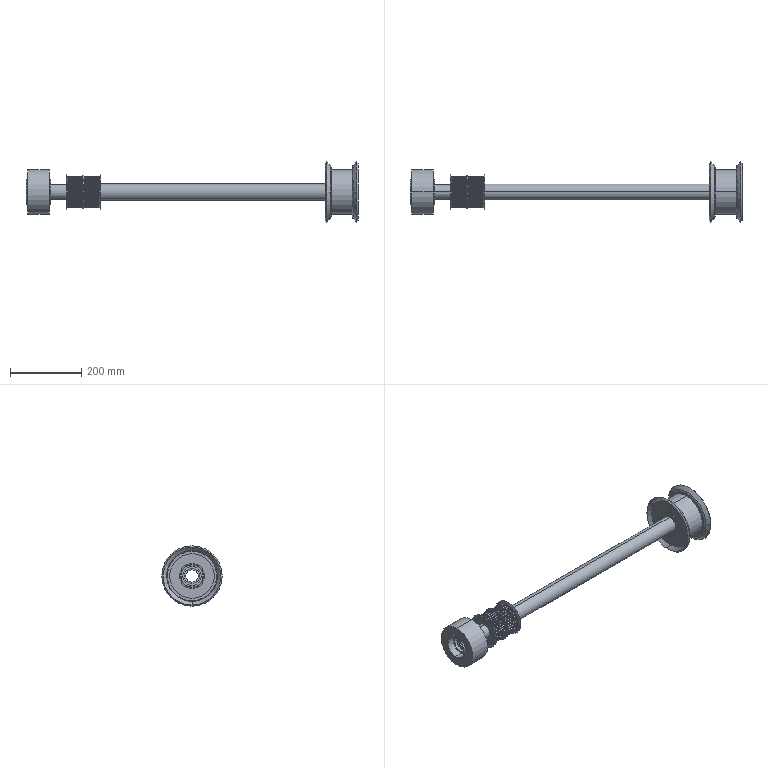Part | SolidWorks | 13 solids | 1456 faces | box 930.556 x 169.042 x 169.042 mm | volume 2373152 mm3 | cylinder 714 | plane 418 | cone 200 | spline 124 | commonest cylinder face diameters 6 x200 1.6 x168 5.14 x168 85.208 x70 5 x16 6.6 x16